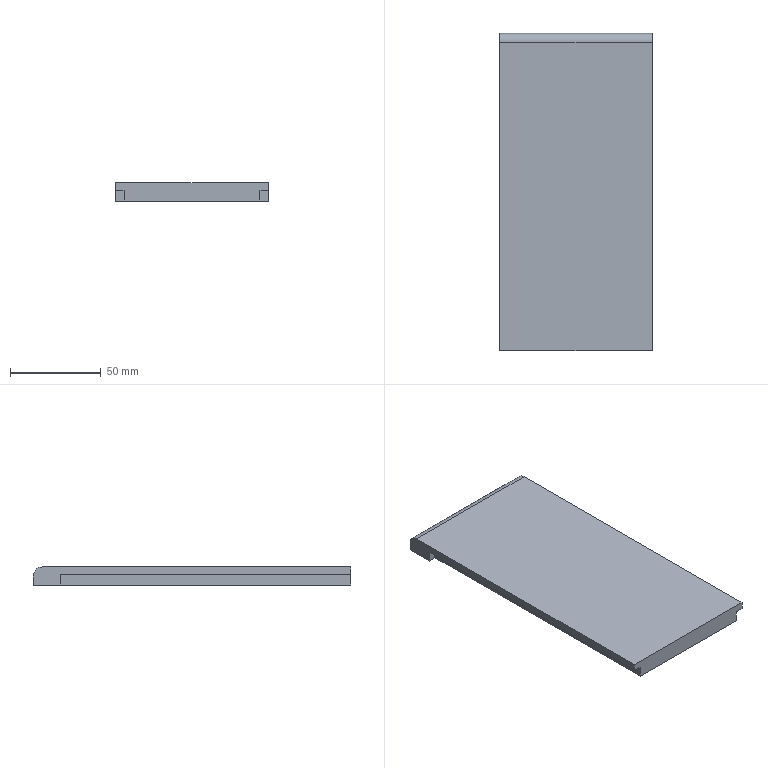Part | STEP file | Head front cover plate | 1 solid | 13 faces | box 84 x 175 x 10 mm | volume 137909 mm3 | plane 12 | cylinder 1 | commonest cylinder face diameters 10 x1
STEP:
#1=CARTESIAN_POINT('',(-42.,95.,48.814));
#2=VERTEX_POINT('',#1);
#3=CARTESIAN_POINT('',(-42.,95.,53.814));
#4=VERTEX_POINT('',#3);
#5=CARTESIAN_POINT('',(-42.,95.,48.814));
#6=DIRECTION('',(0.,0.,1.));
#7=VECTOR('',#6,1000.);
#8=LINE('',#5,#7);
#9=EDGE_CURVE('',#2,#4,#8,.T.);
#10=ORIENTED_EDGE('',*,*,#9,.T.);
#11=CARTESIAN_POINT('',(42.,95.,53.814));
#12=VERTEX_POINT('',#11);
#13=CARTESIAN_POINT('',(-42.,95.,53.814));
#14=DIRECTION('',(1.,0.,0.));
#15=VECTOR('',#14,1000.);
#16=LINE('',#13,#15);
#17=EDGE_CURVE('',#4,#12,#16,.T.);
#18=ORIENTED_EDGE('',*,*,#17,.T.);
#19=CARTESIAN_POINT('',(42.,95.,48.814));
#20=VERTEX_POINT('',#19);
#21=CARTESIAN_POINT('',(42.,95.,48.814));
#22=DIRECTION('',(0.,0.,1.));
#23=VECTOR('',#22,1000.);
#24=LINE('',#21,#23);
#25=EDGE_CURVE('',#20,#12,#24,.T.);
#26=ORIENTED_EDGE('',*,*,#25,.F.);
#27=CARTESIAN_POINT('',(-42.,95.,48.814));
#28=DIRECTION('',(1.,0.,0.));
#29=VECTOR('',#28,1000.);
#30=LINE('',#27,#29);
#31=EDGE_CURVE('',#2,#20,#30,.T.);
#32=ORIENTED_EDGE('',*,*,#31,.F.);
#33=EDGE_LOOP('',(#10,#18,#26,#32));
#34=FACE_OUTER_BOUND('',#33,.T.);
#35=CARTESIAN_POINT('',(-42.,95.,48.814));
#36=DIRECTION('',(0.,1.,0.));
#37=DIRECTION('',(0.,0.,1.));
#38=AXIS2_PLACEMENT_3D('',#35,#36,#37);
#39=PLANE('',#38);
#40=ADVANCED_FACE('',(#34),#39,.T.);
#41=CARTESIAN_POINT('',(-37.5,80.,48.814));
#42=VERTEX_POINT('',#41);
#43=CARTESIAN_POINT('',(-42.,80.,48.814));
#44=VERTEX_POINT('',#43);
#45=CARTESIAN_POINT('',(-37.5,80.,48.814));
#46=DIRECTION('',(-1.,0.,0.));
#47=VECTOR('',#46,1000.);
#48=LINE('',#45,#47);
#49=EDGE_CURVE('',#42,#44,#48,.T.);
#50=ORIENTED_EDGE('',*,*,#49,.T.);
#51=CARTESIAN_POINT('',(-42.,-80.,48.814));
#52=DIRECTION('',(0.,1.,0.));
#53=VECTOR('',#52,1000.);
#54=LINE('',#51,#53);
#55=EDGE_CURVE('',#44,#2,#54,.T.);
#56=ORIENTED_EDGE('',*,*,#55,.T.);
#57=ORIENTED_EDGE('',*,*,#31,.T.);
#58=CARTESIAN_POINT('',(42.,80.,48.814));
#59=VERTEX_POINT('',#58);
#60=CARTESIAN_POINT('',(42.,-80.,48.814));
#61=DIRECTION('',(0.,1.,0.));
#62=VECTOR('',#61,1000.);
#63=LINE('',#60,#62);
#64=EDGE_CURVE('',#59,#20,#63,.T.);
#65=ORIENTED_EDGE('',*,*,#64,.F.);
#66=CARTESIAN_POINT('',(37.5,80.,48.814));
#67=VERTEX_POINT('',#66);
#68=CARTESIAN_POINT('',(37.5,80.,48.814));
#69=DIRECTION('',(1.,0.,0.));
#70=VECTOR('',#69,1000.);
#71=LINE('',#68,#70);
#72=EDGE_CURVE('',#67,#59,#71,.T.);
#73=ORIENTED_EDGE('',*,*,#72,.F.);
#74=CARTESIAN_POINT('',(37.5,-80.,48.814));
#75=VERTEX_POINT('',#74);
#76=CARTESIAN_POINT('',(37.5,-80.,48.814));
#77=DIRECTION('',(0.,1.,0.));
#78=VECTOR('',#77,1000.);
#79=LINE('',#76,#78);
#80=EDGE_CURVE('',#75,#67,#79,.T.);
#81=ORIENTED_EDGE('',*,*,#80,.F.);
#82=CARTESIAN_POINT('',(-37.5,-80.,48.814));
#83=VERTEX_POINT('',#82);
#84=CARTESIAN_POINT('',(-42.,-80.,48.814));
#85=DIRECTION('',(1.,0.,0.));
#86=VECTOR('',#85,1000.);
#87=LINE('',#84,#86);
#88=EDGE_CURVE('',#83,#75,#87,.T.);
#89=ORIENTED_EDGE('',*,*,#88,.F.);
#90=CARTESIAN_POINT('',(-37.5,80.,48.814));
#91=DIRECTION('',(0.,-1.,0.));
#92=VECTOR('',#91,1000.);
#93=LINE('',#90,#92);
#94=EDGE_CURVE('',#42,#83,#93,.T.);
#95=ORIENTED_EDGE('',*,*,#94,.F.);
#96=EDGE_LOOP('',(#50,#56,#57,#65,#73,#81,#89,#95));
#97=FACE_OUTER_BOUND('',#96,.T.);
#98=CARTESIAN_POINT('',(-42.,-80.,48.814));
#99=DIRECTION('',(0.,0.,-1.));
#100=DIRECTION('',(-1.,0.,0.));
#101=AXIS2_PLACEMENT_3D('',#98,#99,#100);
#102=PLANE('',#101);
#103=ADVANCED_FACE('',(#97),#102,.T.);
#104=CARTESIAN_POINT('',(-37.5,-80.,54.814));
#105=VERTEX_POINT('',#104);
#106=CARTESIAN_POINT('',(-42.,-80.,54.814));
#107=VERTEX_POINT('',#106);
#108=CARTESIAN_POINT('',(-37.5,-80.,54.814));
#109=DIRECTION('',(-1.,0.,0.));
#110=VECTOR('',#109,1000.);
#111=LINE('',#108,#110);
#112=EDGE_CURVE('',#105,#107,#111,.T.);
#113=ORIENTED_EDGE('',*,*,#112,.F.);
#114=CARTESIAN_POINT('',(-37.5,-80.,48.814));
#115=DIRECTION('',(0.,0.,1.));
#116=VECTOR('',#115,1000.);
#117=LINE('',#114,#116);
#118=EDGE_CURVE('',#83,#105,#117,.T.);
#119=ORIENTED_EDGE('',*,*,#118,.F.);
#120=ORIENTED_EDGE('',*,*,#88,.T.);
#121=CARTESIAN_POINT('',(37.5,-80.,54.814));
#122=VERTEX_POINT('',#121);
#123=CARTESIAN_POINT('',(37.5,-80.,54.814));
#124=DIRECTION('',(0.,0.,-1.));
#125=VECTOR('',#124,1000.);
#126=LINE('',#123,#125);
#127=EDGE_CURVE('',#122,#75,#126,.T.);
#128=ORIENTED_EDGE('',*,*,#127,.F.);
#129=CARTESIAN_POINT('',(42.,-80.,54.814));
#130=VERTEX_POINT('',#129);
#131=CARTESIAN_POINT('',(37.5,-80.,54.814));
#132=DIRECTION('',(1.,0.,0.));
#133=VECTOR('',#132,1000.);
#134=LINE('',#131,#133);
#135=EDGE_CURVE('',#122,#130,#134,.T.);
#136=ORIENTED_EDGE('',*,*,#135,.T.);
#137=CARTESIAN_POINT('',(42.,-80.,58.814));
#138=VERTEX_POINT('',#137);
#139=CARTESIAN_POINT('',(42.,-80.,58.814));
#140=DIRECTION('',(0.,0.,-1.));
#141=VECTOR('',#140,1000.);
#142=LINE('',#139,#141);
#143=EDGE_CURVE('',#138,#130,#142,.T.);
#144=ORIENTED_EDGE('',*,*,#143,.F.);
#145=CARTESIAN_POINT('',(-42.,-80.,58.814));
#146=VERTEX_POINT('',#145);
#147=CARTESIAN_POINT('',(-42.,-80.,58.814));
#148=DIRECTION('',(1.,0.,0.));
#149=VECTOR('',#148,1000.);
#150=LINE('',#147,#149);
#151=EDGE_CURVE('',#146,#138,#150,.T.);
#152=ORIENTED_EDGE('',*,*,#151,.F.);
#153=CARTESIAN_POINT('',(-42.,-80.,58.814));
#154=DIRECTION('',(0.,0.,-1.));
#155=VECTOR('',#154,1000.);
#156=LINE('',#153,#155);
#157=EDGE_CURVE('',#146,#107,#156,.T.);
#158=ORIENTED_EDGE('',*,*,#157,.T.);
#159=EDGE_LOOP('',(#113,#119,#120,#128,#136,#144,#152,#158));
#160=FACE_OUTER_BOUND('',#159,.T.);
#161=CARTESIAN_POINT('',(-42.,-80.,58.814));
#162=DIRECTION('',(0.,-1.,0.));
#163=DIRECTION('',(0.,0.,-1.));
#164=AXIS2_PLACEMENT_3D('',#161,#162,#163);
#165=PLANE('',#164);
#166=ADVANCED_FACE('',(#160),#165,.T.);
#167=CARTESIAN_POINT('',(42.,90.,58.814));
#168=VERTEX_POINT('',#167);
#169=CARTESIAN_POINT('',(42.,95.,58.814));
#170=DIRECTION('',(0.,-1.,0.));
#171=VECTOR('',#170,1000.);
#172=LINE('',#169,#171);
#173=EDGE_CURVE('',#168,#138,#172,.T.);
#174=ORIENTED_EDGE('',*,*,#173,.F.);
#175=CARTESIAN_POINT('',(-42.,90.,58.814));
#176=VERTEX_POINT('',#175);
#177=CARTESIAN_POINT('',(-42.,90.,58.814));
#178=DIRECTION('',(-1.,0.,0.));
#179=VECTOR('',#178,1000.);
#180=LINE('',#177,#179);
#181=EDGE_CURVE('',#168,#176,#180,.T.);
#182=ORIENTED_EDGE('',*,*,#181,.T.);
#183=CARTESIAN_POINT('',(-42.,95.,58.814));
#184=DIRECTION('',(0.,-1.,0.));
#185=VECTOR('',#184,1000.);
#186=LINE('',#183,#185);
#187=EDGE_CURVE('',#176,#146,#186,.T.);
#188=ORIENTED_EDGE('',*,*,#187,.T.);
#189=ORIENTED_EDGE('',*,*,#151,.T.);
#190=EDGE_LOOP('',(#174,#182,#188,#189));
#191=FACE_OUTER_BOUND('',#190,.T.);
#192=CARTESIAN_POINT('',(-42.,95.,58.814));
#193=DIRECTION('',(0.,0.,1.));
#194=DIRECTION('',(0.,-1.,0.));
#195=AXIS2_PLACEMENT_3D('',#192,#193,#194);
#196=PLANE('',#195);
#197=ADVANCED_FACE('',(#191),#196,.T.);
#198=ORIENTED_EDGE('',*,*,#187,.F.);
#199=CARTESIAN_POINT('',(-42.,90.,53.814));
#200=DIRECTION('',(-1.,0.,0.));
#201=DIRECTION('',(0.,0.,-1.));
#202=AXIS2_PLACEMENT_3D('',#199,#200,#201);
#203=CIRCLE('',#202,5.);
#204=EDGE_CURVE('',#176,#4,#203,.T.);
#205=ORIENTED_EDGE('',*,*,#204,.T.);
#206=ORIENTED_EDGE('',*,*,#9,.F.);
#207=ORIENTED_EDGE('',*,*,#55,.F.);
#208=CARTESIAN_POINT('',(-42.,80.,54.814));
#209=VERTEX_POINT('',#208);
#210=CARTESIAN_POINT('',(-42.,80.,54.814));
#211=DIRECTION('',(0.,0.,-1.));
#212=VECTOR('',#211,1000.);
#213=LINE('',#210,#212);
#214=EDGE_CURVE('',#209,#44,#213,.T.);
#215=ORIENTED_EDGE('',*,*,#214,.F.);
#216=CARTESIAN_POINT('',(-42.,-80.,54.814));
#217=DIRECTION('',(0.,1.,0.));
#218=VECTOR('',#217,1000.);
#219=LINE('',#216,#218);
#220=EDGE_CURVE('',#107,#209,#219,.T.);
#221=ORIENTED_EDGE('',*,*,#220,.F.);
#222=ORIENTED_EDGE('',*,*,#157,.F.);
#223=EDGE_LOOP('',(#198,#205,#206,#207,#215,#221,#222));
#224=FACE_OUTER_BOUND('',#223,.T.);
#225=CARTESIAN_POINT('',(-42.,0.,0.));
#226=DIRECTION('',(1.,0.,0.));
#227=DIRECTION('',(0.,0.,-1.));
#228=AXIS2_PLACEMENT_3D('',#225,#226,#227);
#229=PLANE('',#228);
#230=ADVANCED_FACE('',(#224),#229,.F.);
#231=ORIENTED_EDGE('',*,*,#25,.T.);
#232=CARTESIAN_POINT('',(42.,90.,53.814));
#233=DIRECTION('',(1.,0.,0.));
#234=DIRECTION('',(0.,0.,-1.));
#235=AXIS2_PLACEMENT_3D('',#232,#233,#234);
#236=CIRCLE('',#235,5.);
#237=EDGE_CURVE('',#12,#168,#236,.T.);
#238=ORIENTED_EDGE('',*,*,#237,.T.);
#239=ORIENTED_EDGE('',*,*,#173,.T.);
#240=ORIENTED_EDGE('',*,*,#143,.T.);
#241=CARTESIAN_POINT('',(42.,80.,54.814));
#242=VERTEX_POINT('',#241);
#243=CARTESIAN_POINT('',(42.,80.,54.814));
#244=DIRECTION('',(0.,-1.,0.));
#245=VECTOR('',#244,1000.);
#246=LINE('',#243,#245);
#247=EDGE_CURVE('',#242,#130,#246,.T.);
#248=ORIENTED_EDGE('',*,*,#247,.F.);
#249=CARTESIAN_POINT('',(42.,80.,48.814));
#250=DIRECTION('',(0.,0.,1.));
#251=VECTOR('',#250,1000.);
#252=LINE('',#249,#251);
#253=EDGE_CURVE('',#59,#242,#252,.T.);
#254=ORIENTED_EDGE('',*,*,#253,.F.);
#255=ORIENTED_EDGE('',*,*,#64,.T.);
#256=EDGE_LOOP('',(#231,#238,#239,#240,#248,#254,#255));
#257=FACE_OUTER_BOUND('',#256,.T.);
#258=CARTESIAN_POINT('',(42.,0.,0.));
#259=DIRECTION('',(1.,0.,0.));
#260=DIRECTION('',(0.,0.,-1.));
#261=AXIS2_PLACEMENT_3D('',#258,#259,#260);
#262=PLANE('',#261);
#263=ADVANCED_FACE('',(#257),#262,.T.);
#264=ORIENTED_EDGE('',*,*,#247,.T.);
#265=ORIENTED_EDGE('',*,*,#135,.F.);
#266=CARTESIAN_POINT('',(37.5,80.,54.814));
#267=VERTEX_POINT('',#266);
#268=CARTESIAN_POINT('',(37.5,80.,54.814));
#269=DIRECTION('',(0.,-1.,0.));
#270=VECTOR('',#269,1000.);
#271=LINE('',#268,#270);
#272=EDGE_CURVE('',#267,#122,#271,.T.);
#273=ORIENTED_EDGE('',*,*,#272,.F.);
#274=CARTESIAN_POINT('',(37.5,80.,54.814));
#275=DIRECTION('',(1.,0.,0.));
#276=VECTOR('',#275,1000.);
#277=LINE('',#274,#276);
#278=EDGE_CURVE('',#267,#242,#277,.T.);
#279=ORIENTED_EDGE('',*,*,#278,.T.);
#280=EDGE_LOOP('',(#264,#265,#273,#279));
#281=FACE_OUTER_BOUND('',#280,.T.);
#282=CARTESIAN_POINT('',(37.5,80.,54.814));
#283=DIRECTION('',(0.,0.,1.));
#284=DIRECTION('',(1.,0.,0.));
#285=AXIS2_PLACEMENT_3D('',#282,#283,#284);
#286=PLANE('',#285);
#287=ADVANCED_FACE('',(#281),#286,.F.);
#288=ORIENTED_EDGE('',*,*,#253,.T.);
#289=ORIENTED_EDGE('',*,*,#278,.F.);
#290=CARTESIAN_POINT('',(37.5,80.,48.814));
#291=DIRECTION('',(0.,0.,1.));
#292=VECTOR('',#291,1000.);
#293=LINE('',#290,#292);
#294=EDGE_CURVE('',#67,#267,#293,.T.);
#295=ORIENTED_EDGE('',*,*,#294,.F.);
#296=ORIENTED_EDGE('',*,*,#72,.T.);
#297=EDGE_LOOP('',(#288,#289,#295,#296));
#298=FACE_OUTER_BOUND('',#297,.T.);
#299=CARTESIAN_POINT('',(37.5,80.,48.814));
#300=DIRECTION('',(0.,1.,0.));
#301=DIRECTION('',(-1.,0.,0.));
#302=AXIS2_PLACEMENT_3D('',#299,#300,#301);
#303=PLANE('',#302);
#304=ADVANCED_FACE('',(#298),#303,.F.);
#305=ORIENTED_EDGE('',*,*,#127,.T.);
#306=ORIENTED_EDGE('',*,*,#80,.T.);
#307=ORIENTED_EDGE('',*,*,#294,.T.);
#308=ORIENTED_EDGE('',*,*,#272,.T.);
#309=EDGE_LOOP('',(#305,#306,#307,#308));
#310=FACE_OUTER_BOUND('',#309,.T.);
#311=CARTESIAN_POINT('',(37.5,0.,0.));
#312=DIRECTION('',(1.,0.,0.));
#313=DIRECTION('',(0.,1.,0.));
#314=AXIS2_PLACEMENT_3D('',#311,#312,#313);
#315=PLANE('',#314);
#316=ADVANCED_FACE('',(#310),#315,.T.);
#317=ORIENTED_EDGE('',*,*,#214,.T.);
#318=ORIENTED_EDGE('',*,*,#49,.F.);
#319=CARTESIAN_POINT('',(-37.5,80.,54.814));
#320=VERTEX_POINT('',#319);
#321=CARTESIAN_POINT('',(-37.5,80.,54.814));
#322=DIRECTION('',(0.,0.,-1.));
#323=VECTOR('',#322,1000.);
#324=LINE('',#321,#323);
#325=EDGE_CURVE('',#320,#42,#324,.T.);
#326=ORIENTED_EDGE('',*,*,#325,.F.);
#327=CARTESIAN_POINT('',(-37.5,80.,54.814));
#328=DIRECTION('',(-1.,0.,0.));
#329=VECTOR('',#328,1000.);
#330=LINE('',#327,#329);
#331=EDGE_CURVE('',#320,#209,#330,.T.);
#332=ORIENTED_EDGE('',*,*,#331,.T.);
#333=EDGE_LOOP('',(#317,#318,#326,#332));
#334=FACE_OUTER_BOUND('',#333,.T.);
#335=CARTESIAN_POINT('',(-37.5,80.,54.814));
#336=DIRECTION('',(0.,1.,0.));
#337=DIRECTION('',(-1.,0.,0.));
#338=AXIS2_PLACEMENT_3D('',#335,#336,#337);
#339=PLANE('',#338);
#340=ADVANCED_FACE('',(#334),#339,.F.);
#341=ORIENTED_EDGE('',*,*,#220,.T.);
#342=ORIENTED_EDGE('',*,*,#331,.F.);
#343=CARTESIAN_POINT('',(-37.5,-80.,54.814));
#344=DIRECTION('',(0.,1.,0.));
#345=VECTOR('',#344,1000.);
#346=LINE('',#343,#345);
#347=EDGE_CURVE('',#105,#320,#346,.T.);
#348=ORIENTED_EDGE('',*,*,#347,.F.);
#349=ORIENTED_EDGE('',*,*,#112,.T.);
#350=EDGE_LOOP('',(#341,#342,#348,#349));
#351=FACE_OUTER_BOUND('',#350,.T.);
#352=CARTESIAN_POINT('',(-37.5,-80.,54.814));
#353=DIRECTION('',(0.,0.,1.));
#354=DIRECTION('',(1.,0.,0.));
#355=AXIS2_PLACEMENT_3D('',#352,#353,#354);
#356=PLANE('',#355);
#357=ADVANCED_FACE('',(#351),#356,.F.);
#358=ORIENTED_EDGE('',*,*,#118,.T.);
#359=ORIENTED_EDGE('',*,*,#347,.T.);
#360=ORIENTED_EDGE('',*,*,#325,.T.);
#361=ORIENTED_EDGE('',*,*,#94,.T.);
#362=EDGE_LOOP('',(#358,#359,#360,#361));
#363=FACE_OUTER_BOUND('',#362,.T.);
#364=CARTESIAN_POINT('',(-37.5,0.,0.));
#365=DIRECTION('',(-1.,0.,0.));
#366=DIRECTION('',(0.,-1.,0.));
#367=AXIS2_PLACEMENT_3D('',#364,#365,#366);
#368=PLANE('',#367);
#369=ADVANCED_FACE('',(#363),#368,.T.);
#370=ORIENTED_EDGE('',*,*,#204,.F.);
#371=ORIENTED_EDGE('',*,*,#181,.F.);
#372=ORIENTED_EDGE('',*,*,#237,.F.);
#373=ORIENTED_EDGE('',*,*,#17,.F.);
#374=EDGE_LOOP('',(#370,#371,#372,#373));
#375=FACE_OUTER_BOUND('',#374,.T.);
#376=CARTESIAN_POINT('',(-42.,90.,53.814));
#377=DIRECTION('',(1.,0.,0.));
#378=DIRECTION('',(0.,0.,-1.));
#379=AXIS2_PLACEMENT_3D('',#376,#377,#378);
#380=CYLINDRICAL_SURFACE('',#379,5.);
#381=ADVANCED_FACE('',(#375),#380,.T.);
#382=CLOSED_SHELL('',(#40,#103,#166,#197,#230,#263,#287,#304,#316,#340,#357,#369,#381));
#383=MANIFOLD_SOLID_BREP('',#382);
#384=CARTESIAN_POINT('',(0.,0.,0.));
#385=DIRECTION('',(0.,0.,1.));
#386=DIRECTION('',(1.,0.,0.));
#387=AXIS2_PLACEMENT_3D('',#384,#385,#386);
#388=(LENGTH_UNIT()NAMED_UNIT(*)SI_UNIT(.MILLI.,.METRE.));
#389=UNCERTAINTY_MEASURE_WITH_UNIT(LENGTH_MEASURE(0.00001),#388,'','');
#390=(NAMED_UNIT(*)PLANE_ANGLE_UNIT()SI_UNIT($,.RADIAN.));
#391=(NAMED_UNIT(*)SI_UNIT($,.STERADIAN.)SOLID_ANGLE_UNIT());
#392=(GEOMETRIC_REPRESENTATION_CONTEXT(3)GLOBAL_UNCERTAINTY_ASSIGNED_CONTEXT((#389))GLOBAL_UNIT_ASSIGNED_CONTEXT((#388,#390,#391))REPRESENTATION_CONTEXT('',''));
#393=ADVANCED_BREP_SHAPE_REPRESENTATION('',(#383,#387),#392);